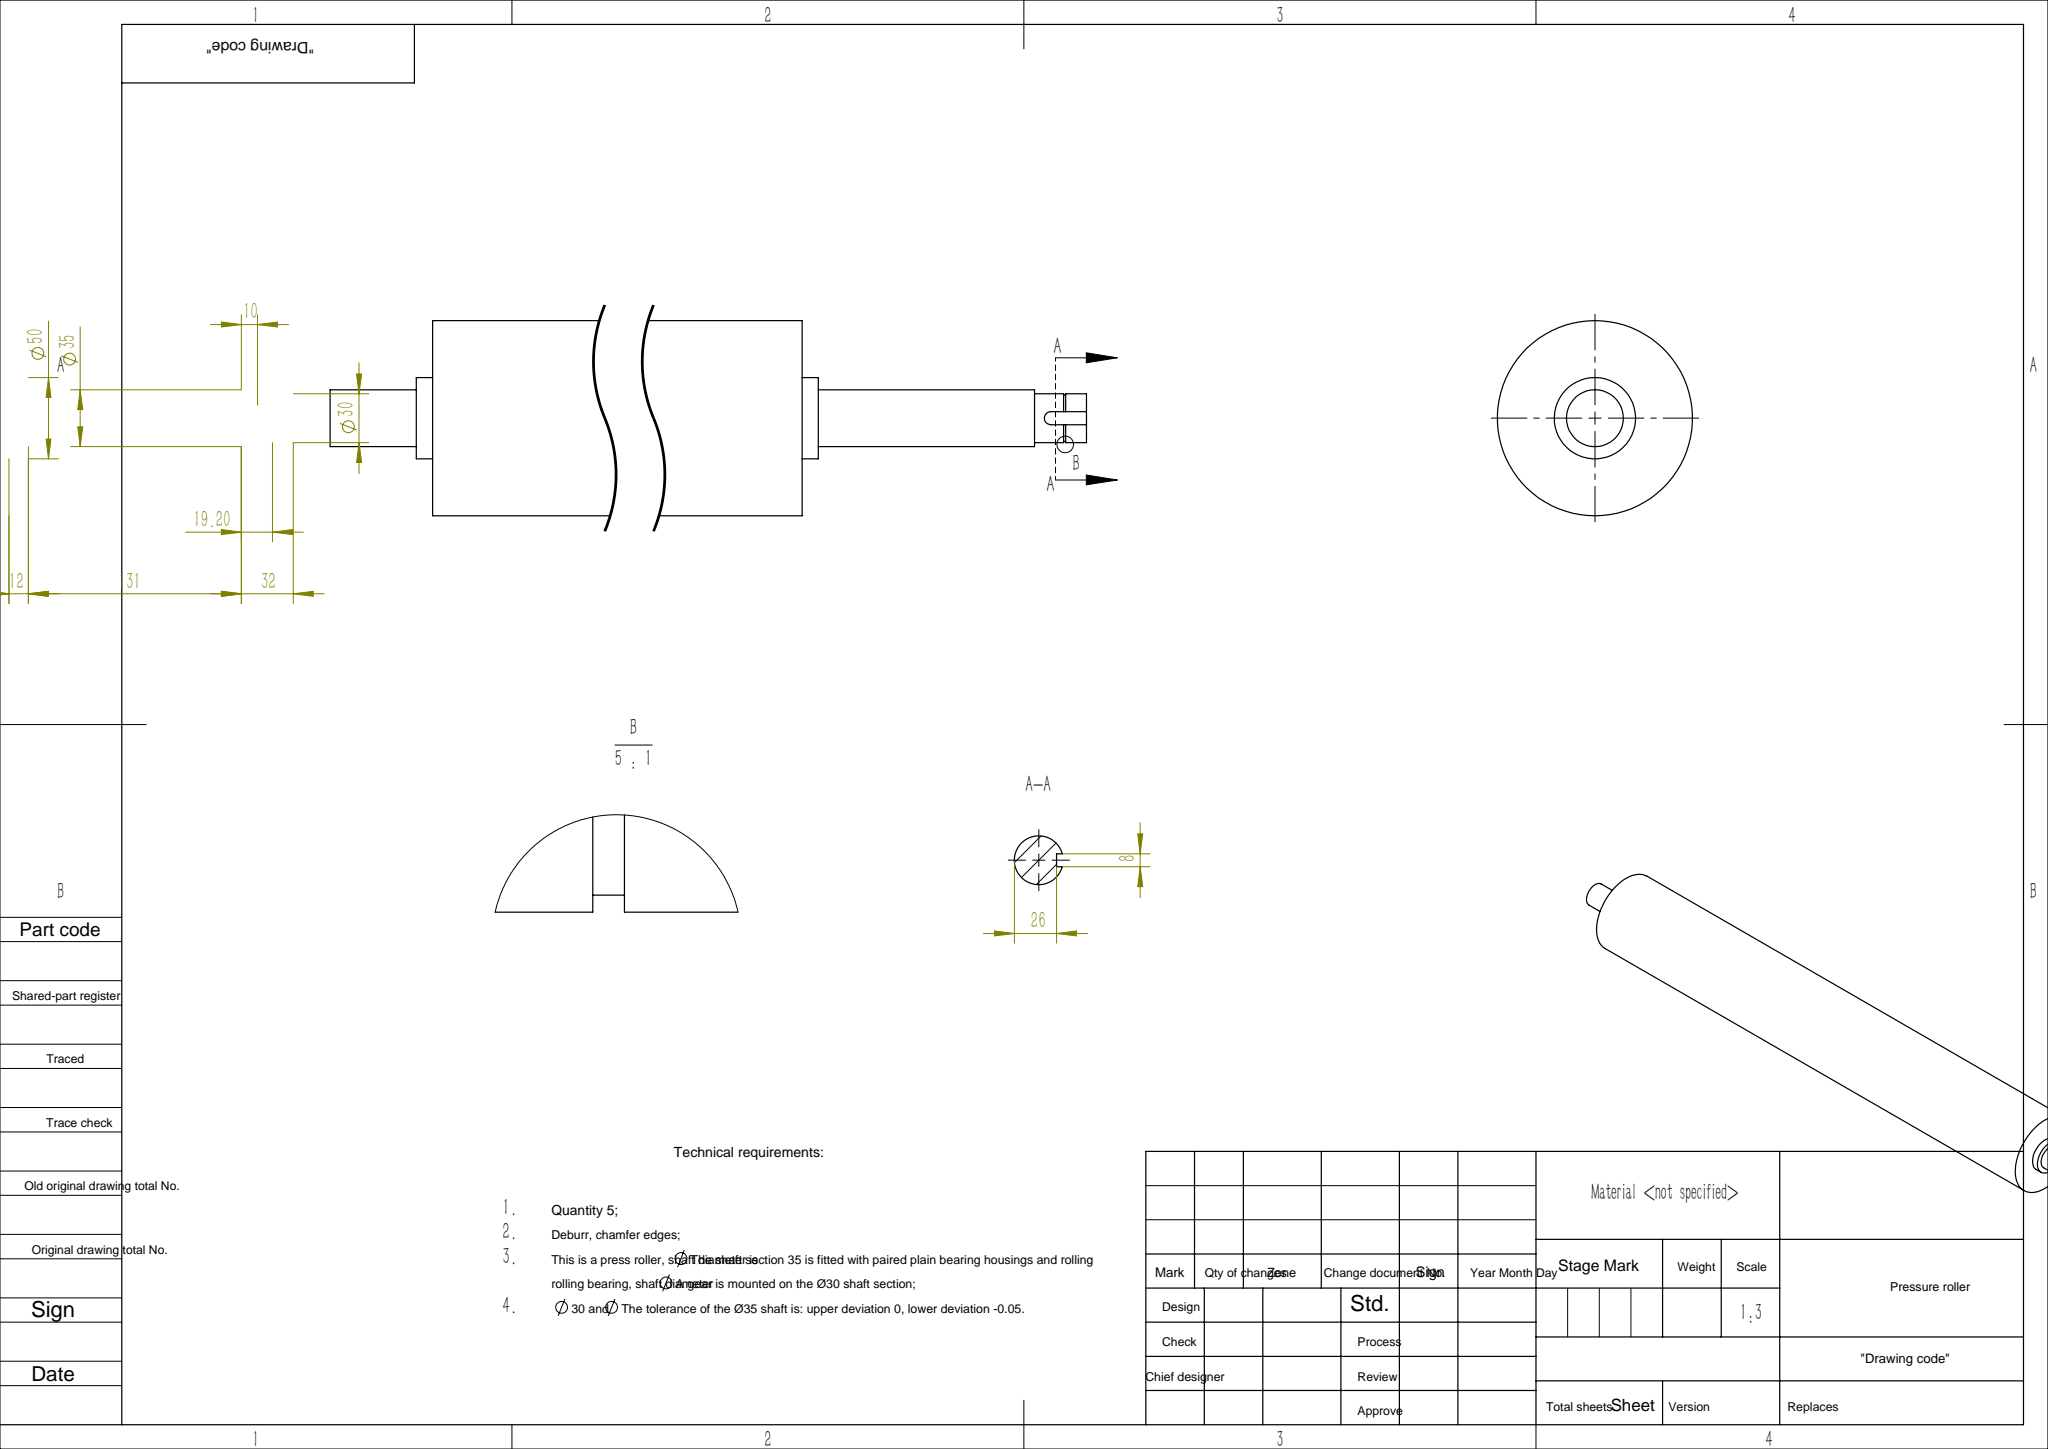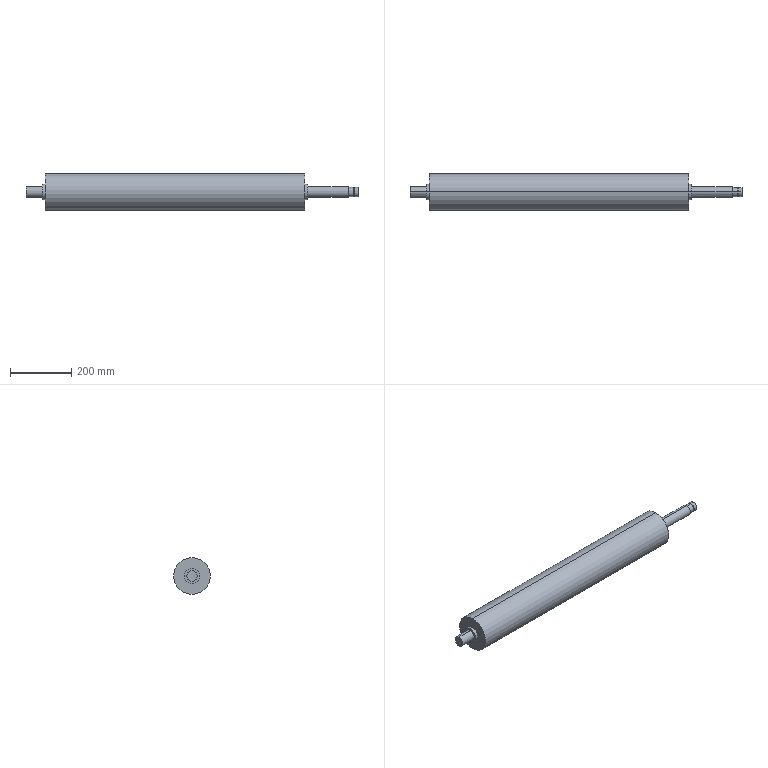Part | SolidWorks | features ICE 2, Revolution 1 | 1 solid | 31 faces | box 1088 x 120 x 120 mm | volume 9853270 mm3 | cylinder 19 | plane 12 | commonest cylinder face diameters 30 x5 35 x4 50 x4 28.6 x3 120 x2 8 x1
STEP:
#1=CARTESIAN_POINT('',(1073.9,13.729,4.));
#2=VERTEX_POINT('',#1);
#3=CARTESIAN_POINT('',(1073.9,0.,14.3));
#4=VERTEX_POINT('',#3);
#5=CARTESIAN_POINT('',(1073.9,0.,0.));
#6=DIRECTION('',(1.,0.,0.));
#7=DIRECTION('',(0.,0.,-1.));
#8=AXIS2_PLACEMENT_3D('',#5,#6,#7);
#9=CIRCLE('',#8,14.3);
#10=EDGE_CURVE('',#2,#4,#9,.T.);
#11=ORIENTED_EDGE('',*,*,#10,.T.);
#12=CARTESIAN_POINT('',(1075.2,0.,14.3));
#13=VERTEX_POINT('',#12);
#14=CARTESIAN_POINT('',(1073.9,0.,14.3));
#15=DIRECTION('',(1.,0.,0.));
#16=VECTOR('',#15,1000.);
#17=LINE('',#14,#16);
#18=EDGE_CURVE('',#4,#13,#17,.T.);
#19=ORIENTED_EDGE('',*,*,#18,.T.);
#20=CARTESIAN_POINT('',(1075.2,13.729,4.));
#21=VERTEX_POINT('',#20);
#22=CARTESIAN_POINT('',(1075.2,0.,0.));
#23=DIRECTION('',(1.,0.,0.));
#24=DIRECTION('',(0.,0.,-1.));
#25=AXIS2_PLACEMENT_3D('',#22,#23,#24);
#26=CIRCLE('',#25,14.3);
#27=EDGE_CURVE('',#21,#13,#26,.T.);
#28=ORIENTED_EDGE('',*,*,#27,.F.);
#29=CARTESIAN_POINT('',(1073.9,13.729,4.));
#30=DIRECTION('',(-1.,0.,0.));
#31=VECTOR('',#30,1000.);
#32=LINE('',#29,#31);
#33=EDGE_CURVE('',#21,#2,#32,.T.);
#34=ORIENTED_EDGE('',*,*,#33,.T.);
#35=EDGE_LOOP('',(#11,#19,#28,#34));
#36=FACE_OUTER_BOUND('',#35,.T.);
#37=CARTESIAN_POINT('',(1073.9,0.,0.));
#38=DIRECTION('',(1.,0.,0.));
#39=DIRECTION('',(0.,0.,-1.));
#40=AXIS2_PLACEMENT_3D('',#37,#38,#39);
#41=CYLINDRICAL_SURFACE('',#40,14.3);
#42=ADVANCED_FACE('',(#36),#41,.T.);
#43=ORIENTED_EDGE('',*,*,#18,.F.);
#44=CARTESIAN_POINT('',(1073.9,0.,-14.3));
#45=VERTEX_POINT('',#44);
#46=CARTESIAN_POINT('',(1073.9,0.,0.));
#47=DIRECTION('',(1.,0.,0.));
#48=DIRECTION('',(0.,0.,-1.));
#49=AXIS2_PLACEMENT_3D('',#46,#47,#48);
#50=CIRCLE('',#49,14.3);
#51=EDGE_CURVE('',#4,#45,#50,.T.);
#52=ORIENTED_EDGE('',*,*,#51,.T.);
#53=CARTESIAN_POINT('',(1075.2,0.,-14.3));
#54=VERTEX_POINT('',#53);
#55=CARTESIAN_POINT('',(1073.9,0.,-14.3));
#56=DIRECTION('',(1.,0.,0.));
#57=VECTOR('',#56,1000.);
#58=LINE('',#55,#57);
#59=EDGE_CURVE('',#45,#54,#58,.T.);
#60=ORIENTED_EDGE('',*,*,#59,.T.);
#61=CARTESIAN_POINT('',(1075.2,0.,0.));
#62=DIRECTION('',(1.,0.,0.));
#63=DIRECTION('',(0.,0.,-1.));
#64=AXIS2_PLACEMENT_3D('',#61,#62,#63);
#65=CIRCLE('',#64,14.3);
#66=EDGE_CURVE('',#13,#54,#65,.T.);
#67=ORIENTED_EDGE('',*,*,#66,.F.);
#68=EDGE_LOOP('',(#43,#52,#60,#67));
#69=FACE_OUTER_BOUND('',#68,.T.);
#70=CARTESIAN_POINT('',(1073.9,0.,0.));
#71=DIRECTION('',(1.,0.,0.));
#72=DIRECTION('',(0.,0.,-1.));
#73=AXIS2_PLACEMENT_3D('',#70,#71,#72);
#74=CYLINDRICAL_SURFACE('',#73,14.3);
#75=ADVANCED_FACE('',(#69),#74,.T.);
#76=CARTESIAN_POINT('',(53.,0.,-25.));
#77=VERTEX_POINT('',#76);
#78=CARTESIAN_POINT('',(53.,0.,25.));
#79=VERTEX_POINT('',#78);
#80=CARTESIAN_POINT('',(53.,0.,0.));
#81=DIRECTION('',(1.,0.,0.));
#82=DIRECTION('',(0.,0.,-1.));
#83=AXIS2_PLACEMENT_3D('',#80,#81,#82);
#84=CIRCLE('',#83,25.);
#85=EDGE_CURVE('',#77,#79,#84,.T.);
#86=ORIENTED_EDGE('',*,*,#85,.T.);
#87=CARTESIAN_POINT('',(63.,0.,25.));
#88=VERTEX_POINT('',#87);
#89=CARTESIAN_POINT('',(1088.,0.,25.));
#90=DIRECTION('',(1.,0.,0.));
#91=VECTOR('',#90,1000.);
#92=LINE('',#89,#91);
#93=EDGE_CURVE('',#79,#88,#92,.T.);
#94=ORIENTED_EDGE('',*,*,#93,.T.);
#95=CARTESIAN_POINT('',(63.,0.,-25.));
#96=VERTEX_POINT('',#95);
#97=CARTESIAN_POINT('',(63.,0.,0.));
#98=DIRECTION('',(1.,0.,0.));
#99=DIRECTION('',(0.,0.,-1.));
#100=AXIS2_PLACEMENT_3D('',#97,#98,#99);
#101=CIRCLE('',#100,25.);
#102=EDGE_CURVE('',#96,#88,#101,.T.);
#103=ORIENTED_EDGE('',*,*,#102,.F.);
#104=CARTESIAN_POINT('',(1088.,0.,-25.));
#105=DIRECTION('',(1.,0.,0.));
#106=VECTOR('',#105,1000.);
#107=LINE('',#104,#106);
#108=EDGE_CURVE('',#77,#96,#107,.T.);
#109=ORIENTED_EDGE('',*,*,#108,.F.);
#110=EDGE_LOOP('',(#86,#94,#103,#109));
#111=FACE_OUTER_BOUND('',#110,.T.);
#112=CARTESIAN_POINT('',(1088.,0.,0.));
#113=DIRECTION('',(1.,0.,0.));
#114=DIRECTION('',(0.,0.,-1.));
#115=AXIS2_PLACEMENT_3D('',#112,#113,#114);
#116=CYLINDRICAL_SURFACE('',#115,25.);
#117=ADVANCED_FACE('',(#111),#116,.T.);
#118=CARTESIAN_POINT('',(63.,0.,-60.));
#119=VERTEX_POINT('',#118);
#120=CARTESIAN_POINT('',(63.,0.,60.));
#121=VERTEX_POINT('',#120);
#122=CARTESIAN_POINT('',(63.,0.,0.));
#123=DIRECTION('',(1.,0.,0.));
#124=DIRECTION('',(0.,0.,-1.));
#125=AXIS2_PLACEMENT_3D('',#122,#123,#124);
#126=CIRCLE('',#125,60.);
#127=EDGE_CURVE('',#119,#121,#126,.T.);
#128=ORIENTED_EDGE('',*,*,#127,.T.);
#129=CARTESIAN_POINT('',(913.,0.,60.));
#130=VERTEX_POINT('',#129);
#131=CARTESIAN_POINT('',(1088.,0.,60.));
#132=DIRECTION('',(1.,0.,0.));
#133=VECTOR('',#132,1000.);
#134=LINE('',#131,#133);
#135=EDGE_CURVE('',#121,#130,#134,.T.);
#136=ORIENTED_EDGE('',*,*,#135,.T.);
#137=CARTESIAN_POINT('',(913.,0.,-60.));
#138=VERTEX_POINT('',#137);
#139=CARTESIAN_POINT('',(913.,0.,0.));
#140=DIRECTION('',(1.,0.,0.));
#141=DIRECTION('',(0.,0.,-1.));
#142=AXIS2_PLACEMENT_3D('',#139,#140,#141);
#143=CIRCLE('',#142,60.);
#144=EDGE_CURVE('',#138,#130,#143,.T.);
#145=ORIENTED_EDGE('',*,*,#144,.F.);
#146=CARTESIAN_POINT('',(1088.,0.,-60.));
#147=DIRECTION('',(1.,0.,0.));
#148=VECTOR('',#147,1000.);
#149=LINE('',#146,#148);
#150=EDGE_CURVE('',#119,#138,#149,.T.);
#151=ORIENTED_EDGE('',*,*,#150,.F.);
#152=EDGE_LOOP('',(#128,#136,#145,#151));
#153=FACE_OUTER_BOUND('',#152,.T.);
#154=CARTESIAN_POINT('',(1088.,0.,0.));
#155=DIRECTION('',(1.,0.,0.));
#156=DIRECTION('',(0.,0.,-1.));
#157=AXIS2_PLACEMENT_3D('',#154,#155,#156);
#158=CYLINDRICAL_SURFACE('',#157,60.);
#159=ADVANCED_FACE('',(#153),#158,.T.);
#160=CARTESIAN_POINT('',(913.,0.,-25.));
#161=VERTEX_POINT('',#160);
#162=CARTESIAN_POINT('',(913.,0.,25.));
#163=VERTEX_POINT('',#162);
#164=CARTESIAN_POINT('',(913.,0.,0.));
#165=DIRECTION('',(1.,0.,0.));
#166=DIRECTION('',(0.,0.,-1.));
#167=AXIS2_PLACEMENT_3D('',#164,#165,#166);
#168=CIRCLE('',#167,25.);
#169=EDGE_CURVE('',#161,#163,#168,.T.);
#170=ORIENTED_EDGE('',*,*,#169,.T.);
#171=CARTESIAN_POINT('',(923.,0.,25.));
#172=VERTEX_POINT('',#171);
#173=CARTESIAN_POINT('',(1088.,0.,25.));
#174=DIRECTION('',(1.,0.,0.));
#175=VECTOR('',#174,1000.);
#176=LINE('',#173,#175);
#177=EDGE_CURVE('',#163,#172,#176,.T.);
#178=ORIENTED_EDGE('',*,*,#177,.T.);
#179=CARTESIAN_POINT('',(923.,0.,-25.));
#180=VERTEX_POINT('',#179);
#181=CARTESIAN_POINT('',(923.,0.,0.));
#182=DIRECTION('',(1.,0.,0.));
#183=DIRECTION('',(0.,0.,-1.));
#184=AXIS2_PLACEMENT_3D('',#181,#182,#183);
#185=CIRCLE('',#184,25.);
#186=EDGE_CURVE('',#180,#172,#185,.T.);
#187=ORIENTED_EDGE('',*,*,#186,.F.);
#188=CARTESIAN_POINT('',(1088.,0.,-25.));
#189=DIRECTION('',(1.,0.,0.));
#190=VECTOR('',#189,1000.);
#191=LINE('',#188,#190);
#192=EDGE_CURVE('',#161,#180,#191,.T.);
#193=ORIENTED_EDGE('',*,*,#192,.F.);
#194=EDGE_LOOP('',(#170,#178,#187,#193));
#195=FACE_OUTER_BOUND('',#194,.T.);
#196=CARTESIAN_POINT('',(1088.,0.,0.));
#197=DIRECTION('',(1.,0.,0.));
#198=DIRECTION('',(0.,0.,-1.));
#199=AXIS2_PLACEMENT_3D('',#196,#197,#198);
#200=CYLINDRICAL_SURFACE('',#199,25.);
#201=ADVANCED_FACE('',(#195),#200,.T.);
#202=CARTESIAN_POINT('',(923.,0.,-17.5));
#203=VERTEX_POINT('',#202);
#204=CARTESIAN_POINT('',(923.,0.,17.5));
#205=VERTEX_POINT('',#204);
#206=CARTESIAN_POINT('',(923.,0.,0.));
#207=DIRECTION('',(1.,0.,0.));
#208=DIRECTION('',(0.,0.,-1.));
#209=AXIS2_PLACEMENT_3D('',#206,#207,#208);
#210=CIRCLE('',#209,17.5);
#211=EDGE_CURVE('',#203,#205,#210,.T.);
#212=ORIENTED_EDGE('',*,*,#211,.T.);
#213=CARTESIAN_POINT('',(1056.,0.,17.5));
#214=VERTEX_POINT('',#213);
#215=CARTESIAN_POINT('',(1088.,0.,17.5));
#216=DIRECTION('',(1.,0.,0.));
#217=VECTOR('',#216,1000.);
#218=LINE('',#215,#217);
#219=EDGE_CURVE('',#205,#214,#218,.T.);
#220=ORIENTED_EDGE('',*,*,#219,.T.);
#221=CARTESIAN_POINT('',(1056.,0.,-17.5));
#222=VERTEX_POINT('',#221);
#223=CARTESIAN_POINT('',(1056.,0.,0.));
#224=DIRECTION('',(1.,0.,0.));
#225=DIRECTION('',(0.,0.,-1.));
#226=AXIS2_PLACEMENT_3D('',#223,#224,#225);
#227=CIRCLE('',#226,17.5);
#228=EDGE_CURVE('',#222,#214,#227,.T.);
#229=ORIENTED_EDGE('',*,*,#228,.F.);
#230=CARTESIAN_POINT('',(1088.,0.,-17.5));
#231=DIRECTION('',(1.,0.,0.));
#232=VECTOR('',#231,1000.);
#233=LINE('',#230,#232);
#234=EDGE_CURVE('',#203,#222,#233,.T.);
#235=ORIENTED_EDGE('',*,*,#234,.F.);
#236=EDGE_LOOP('',(#212,#220,#229,#235));
#237=FACE_OUTER_BOUND('',#236,.T.);
#238=CARTESIAN_POINT('',(1088.,0.,0.));
#239=DIRECTION('',(1.,0.,0.));
#240=DIRECTION('',(0.,0.,-1.));
#241=AXIS2_PLACEMENT_3D('',#238,#239,#240);
#242=CYLINDRICAL_SURFACE('',#241,17.5);
#243=ADVANCED_FACE('',(#237),#242,.T.);
#244=CARTESIAN_POINT('',(1075.2,14.457,4.));
#245=VERTEX_POINT('',#244);
#246=CARTESIAN_POINT('',(1075.2,0.,15.));
#247=VERTEX_POINT('',#246);
#248=CARTESIAN_POINT('',(1075.2,0.,0.));
#249=DIRECTION('',(1.,0.,0.));
#250=DIRECTION('',(0.,0.,-1.));
#251=AXIS2_PLACEMENT_3D('',#248,#249,#250);
#252=CIRCLE('',#251,15.);
#253=EDGE_CURVE('',#245,#247,#252,.T.);
#254=ORIENTED_EDGE('',*,*,#253,.T.);
#255=CARTESIAN_POINT('',(1088.,0.,15.));
#256=VERTEX_POINT('',#255);
#257=CARTESIAN_POINT('',(1088.,0.,15.));
#258=DIRECTION('',(1.,0.,0.));
#259=VECTOR('',#258,1000.);
#260=LINE('',#257,#259);
#261=EDGE_CURVE('',#247,#256,#260,.T.);
#262=ORIENTED_EDGE('',*,*,#261,.T.);
#263=CARTESIAN_POINT('',(1088.,14.457,4.));
#264=VERTEX_POINT('',#263);
#265=CARTESIAN_POINT('',(1088.,0.,0.));
#266=DIRECTION('',(1.,0.,0.));
#267=DIRECTION('',(0.,0.,-1.));
#268=AXIS2_PLACEMENT_3D('',#265,#266,#267);
#269=CIRCLE('',#268,15.);
#270=EDGE_CURVE('',#264,#256,#269,.T.);
#271=ORIENTED_EDGE('',*,*,#270,.F.);
#272=CARTESIAN_POINT('',(1088.,14.457,4.));
#273=DIRECTION('',(1.,0.,0.));
#274=VECTOR('',#273,1000.);
#275=LINE('',#272,#274);
#276=EDGE_CURVE('',#245,#264,#275,.T.);
#277=ORIENTED_EDGE('',*,*,#276,.F.);
#278=EDGE_LOOP('',(#254,#262,#271,#277));
#279=FACE_OUTER_BOUND('',#278,.T.);
#280=CARTESIAN_POINT('',(1088.,0.,0.));
#281=DIRECTION('',(1.,0.,0.));
#282=DIRECTION('',(0.,0.,-1.));
#283=AXIS2_PLACEMENT_3D('',#280,#281,#282);
#284=CYLINDRICAL_SURFACE('',#283,15.);
#285=ADVANCED_FACE('',(#279),#284,.T.);
#286=ORIENTED_EDGE('',*,*,#261,.F.);
#287=CARTESIAN_POINT('',(1075.2,0.,-15.));
#288=VERTEX_POINT('',#287);
#289=CARTESIAN_POINT('',(1075.2,0.,0.));
#290=DIRECTION('',(1.,0.,0.));
#291=DIRECTION('',(0.,0.,-1.));
#292=AXIS2_PLACEMENT_3D('',#289,#290,#291);
#293=CIRCLE('',#292,15.);
#294=EDGE_CURVE('',#247,#288,#293,.T.);
#295=ORIENTED_EDGE('',*,*,#294,.T.);
#296=CARTESIAN_POINT('',(1088.,0.,-15.));
#297=VERTEX_POINT('',#296);
#298=CARTESIAN_POINT('',(1088.,0.,-15.));
#299=DIRECTION('',(1.,0.,0.));
#300=VECTOR('',#299,1000.);
#301=LINE('',#298,#300);
#302=EDGE_CURVE('',#288,#297,#301,.T.);
#303=ORIENTED_EDGE('',*,*,#302,.T.);
#304=CARTESIAN_POINT('',(1088.,0.,0.));
#305=DIRECTION('',(1.,0.,0.));
#306=DIRECTION('',(0.,0.,-1.));
#307=AXIS2_PLACEMENT_3D('',#304,#305,#306);
#308=CIRCLE('',#307,15.);
#309=EDGE_CURVE('',#256,#297,#308,.T.);
#310=ORIENTED_EDGE('',*,*,#309,.F.);
#311=EDGE_LOOP('',(#286,#295,#303,#310));
#312=FACE_OUTER_BOUND('',#311,.T.);
#313=CARTESIAN_POINT('',(1088.,0.,0.));
#314=DIRECTION('',(1.,0.,0.));
#315=DIRECTION('',(0.,0.,-1.));
#316=AXIS2_PLACEMENT_3D('',#313,#314,#315);
#317=CYLINDRICAL_SURFACE('',#316,15.);
#318=ADVANCED_FACE('',(#312),#317,.T.);
#319=CARTESIAN_POINT('',(0.,0.,-17.5));
#320=VERTEX_POINT('',#319);
#321=CARTESIAN_POINT('',(0.,0.,17.5));
#322=VERTEX_POINT('',#321);
#323=CARTESIAN_POINT('',(0.,0.,0.));
#324=DIRECTION('',(1.,0.,0.));
#325=DIRECTION('',(0.,0.,-1.));
#326=AXIS2_PLACEMENT_3D('',#323,#324,#325);
#327=CIRCLE('',#326,17.5);
#328=EDGE_CURVE('',#320,#322,#327,.T.);
#329=ORIENTED_EDGE('',*,*,#328,.T.);
#330=CARTESIAN_POINT('',(53.,0.,17.5));
#331=VERTEX_POINT('',#330);
#332=CARTESIAN_POINT('',(1088.,0.,17.5));
#333=DIRECTION('',(1.,0.,0.));
#334=VECTOR('',#333,1000.);
#335=LINE('',#332,#334);
#336=EDGE_CURVE('',#322,#331,#335,.T.);
#337=ORIENTED_EDGE('',*,*,#336,.T.);
#338=CARTESIAN_POINT('',(53.,0.,-17.5));
#339=VERTEX_POINT('',#338);
#340=CARTESIAN_POINT('',(53.,0.,0.));
#341=DIRECTION('',(1.,0.,0.));
#342=DIRECTION('',(0.,0.,-1.));
#343=AXIS2_PLACEMENT_3D('',#340,#341,#342);
#344=CIRCLE('',#343,17.5);
#345=EDGE_CURVE('',#339,#331,#344,.T.);
#346=ORIENTED_EDGE('',*,*,#345,.F.);
#347=CARTESIAN_POINT('',(1088.,0.,-17.5));
#348=DIRECTION('',(1.,0.,0.));
#349=VECTOR('',#348,1000.);
#350=LINE('',#347,#349);
#351=EDGE_CURVE('',#320,#339,#350,.T.);
#352=ORIENTED_EDGE('',*,*,#351,.F.);
#353=EDGE_LOOP('',(#329,#337,#346,#352));
#354=FACE_OUTER_BOUND('',#353,.T.);
#355=CARTESIAN_POINT('',(1088.,0.,0.));
#356=DIRECTION('',(1.,0.,0.));
#357=DIRECTION('',(0.,0.,-1.));
#358=AXIS2_PLACEMENT_3D('',#355,#356,#357);
#359=CYLINDRICAL_SURFACE('',#358,17.5);
#360=ADVANCED_FACE('',(#354),#359,.T.);
#361=CARTESIAN_POINT('',(1056.,0.,-15.));
#362=VERTEX_POINT('',#361);
#363=CARTESIAN_POINT('',(1056.,0.,15.));
#364=VERTEX_POINT('',#363);
#365=CARTESIAN_POINT('',(1056.,0.,0.));
#366=DIRECTION('',(1.,0.,0.));
#367=DIRECTION('',(0.,0.,-1.));
#368=AXIS2_PLACEMENT_3D('',#365,#366,#367);
#369=CIRCLE('',#368,15.);
#370=EDGE_CURVE('',#362,#364,#369,.T.);
#371=ORIENTED_EDGE('',*,*,#370,.T.);
#372=CARTESIAN_POINT('',(1073.9,0.,15.));
#373=VERTEX_POINT('',#372);
#374=CARTESIAN_POINT('',(1088.,0.,15.));
#375=DIRECTION('',(1.,0.,0.));
#376=VECTOR('',#375,1000.);
#377=LINE('',#374,#376);
#378=EDGE_CURVE('',#364,#373,#377,.T.);
#379=ORIENTED_EDGE('',*,*,#378,.T.);
#380=CARTESIAN_POINT('',(1073.9,14.457,4.));
#381=VERTEX_POINT('',#380);
#382=CARTESIAN_POINT('',(1073.9,0.,0.));
#383=DIRECTION('',(1.,0.,0.));
#384=DIRECTION('',(0.,0.,-1.));
#385=AXIS2_PLACEMENT_3D('',#382,#383,#384);
#386=CIRCLE('',#385,15.);
#387=EDGE_CURVE('',#381,#373,#386,.T.);
#388=ORIENTED_EDGE('',*,*,#387,.F.);
#389=CARTESIAN_POINT('',(1066.,14.457,4.));
#390=VERTEX_POINT('',#389);
#391=CARTESIAN_POINT('',(1088.,14.457,4.));
#392=DIRECTION('',(1.,0.,0.));
#393=VECTOR('',#392,1000.);
#394=LINE('',#391,#393);
#395=EDGE_CURVE('',#390,#381,#394,.T.);
#396=ORIENTED_EDGE('',*,*,#395,.F.);
#397=CARTESIAN_POINT('',(1066.,14.457,-4.));
#398=VERTEX_POINT('',#397);
#399=CARTESIAN_POINT('',(1066.,14.457,-4.));
#400=CARTESIAN_POINT('',(1065.734,14.457,-4.));
#401=CARTESIAN_POINT('',(1065.474,14.464,-3.974));
#402=CARTESIAN_POINT('',(1064.961,14.492,-3.872));
#403=CARTESIAN_POINT('',(1064.706,14.513,-3.794));
#404=CARTESIAN_POINT('',(1064.223,14.564,-3.593));
#405=CARTESIAN_POINT('',(1063.993,14.594,-3.47));
#406=CARTESIAN_POINT('',(1063.56,14.66,-3.18));
#407=CARTESIAN_POINT('',(1063.355,14.696,-3.012));
#408=CARTESIAN_POINT('',(1062.988,14.766,-2.645));
#409=CARTESIAN_POINT('',(1062.823,14.801,-2.444));
#410=CARTESIAN_POINT('',(1062.53,14.867,-2.008));
#411=CARTESIAN_POINT('',(1062.407,14.896,-1.777));
#412=CARTESIAN_POINT('',(1062.207,14.946,-1.296));
#413=CARTESIAN_POINT('',(1062.129,14.966,-1.043));
#414=CARTESIAN_POINT('',(1062.026,14.993,-0.5261));
#415=CARTESIAN_POINT('',(1062.,15.,-0.2658));
#416=CARTESIAN_POINT('',(1062.,15.,0.2585));
#417=CARTESIAN_POINT('',(1062.026,14.993,0.5249));
#418=CARTESIAN_POINT('',(1062.128,14.966,1.039));
#419=CARTESIAN_POINT('',(1062.204,14.947,1.289));
#420=CARTESIAN_POINT('',(1062.506,14.872,2.017));
#421=CARTESIAN_POINT('',(1062.801,14.802,2.457));
#422=CARTESIAN_POINT('',(1063.355,14.696,3.012));
#423=CARTESIAN_POINT('',(1063.556,14.66,3.177));
#424=CARTESIAN_POINT('',(1063.988,14.595,3.467));
#425=CARTESIAN_POINT('',(1064.222,14.564,3.593));
#426=CARTESIAN_POINT('',(1064.704,14.513,3.793));
#427=CARTESIAN_POINT('',(1064.954,14.492,3.87));
#428=CARTESIAN_POINT('',(1065.469,14.464,3.973));
#429=CARTESIAN_POINT('',(1065.734,14.457,4.));
#430=CARTESIAN_POINT('',(1066.,14.457,4.));
#431=B_SPLINE_CURVE_WITH_KNOTS('',3,(#399,#400,#401,#402,#403,#404,#405,#406,#407,#408,#409,#410,#411,#412,#413,#414,#415,#416,#417,#418,#419,#420,#421,#422,#423,#424,#425,#426,#427,#428,#429,#430),.UNSPECIFIED.,.F.,.F.,(4,2,2,2,2,2,2,2,2,2,2,2,2,2,2,4),(0.,0.0007849,0.00157,0.002355,0.00314,0.003925,0.00471,0.005494,0.006279,0.007064,0.007849,0.009419,0.0102,0.01099,0.01177,0.01256),.UNSPECIFIED.);
#432=EDGE_CURVE('',#398,#390,#431,.T.);
#433=ORIENTED_EDGE('',*,*,#432,.F.);
#434=CARTESIAN_POINT('',(1073.9,14.457,-4.));
#435=VERTEX_POINT('',#434);
#436=CARTESIAN_POINT('',(1088.,14.457,-4.));
#437=DIRECTION('',(-1.,0.,0.));
#438=VECTOR('',#437,1000.);
#439=LINE('',#436,#438);
#440=EDGE_CURVE('',#435,#398,#439,.T.);
#441=ORIENTED_EDGE('',*,*,#440,.F.);
#442=CARTESIAN_POINT('',(1073.9,0.,-15.));
#443=VERTEX_POINT('',#442);
#444=CARTESIAN_POINT('',(1073.9,0.,0.));
#445=DIRECTION('',(1.,0.,0.));
#446=DIRECTION('',(0.,0.,-1.));
#447=AXIS2_PLACEMENT_3D('',#444,#445,#446);
#448=CIRCLE('',#447,15.);
#449=EDGE_CURVE('',#443,#435,#448,.T.);
#450=ORIENTED_EDGE('',*,*,#449,.F.);
#451=CARTESIAN_POINT('',(1088.,0.,-15.));
#452=DIRECTION('',(1.,0.,0.));
#453=VECTOR('',#452,1000.);
#454=LINE('',#451,#453);
#455=EDGE_CURVE('',#362,#443,#454,.T.);
#456=ORIENTED_EDGE('',*,*,#455,.F.);
#457=EDGE_LOOP('',(#371,#379,#388,#396,#433,#441,#450,#456));
#458=FACE_OUTER_BOUND('',#457,.T.);
#459=CARTESIAN_POINT('',(1088.,0.,0.));
#460=DIRECTION('',(1.,0.,0.));
#461=DIRECTION('',(0.,0.,-1.));
#462=AXIS2_PLACEMENT_3D('',#459,#460,#461);
#463=CYLINDRICAL_SURFACE('',#462,15.);
#464=ADVANCED_FACE('',(#458),#463,.T.);
#465=ORIENTED_EDGE('',*,*,#378,.F.);
#466=CARTESIAN_POINT('',(1056.,0.,0.));
#467=DIRECTION('',(1.,0.,0.));
#468=DIRECTION('',(0.,0.,-1.));
#469=AXIS2_PLACEMENT_3D('',#466,#467,#468);
#470=CIRCLE('',#469,15.);
#471=EDGE_CURVE('',#364,#362,#470,.T.);
#472=ORIENTED_EDGE('',*,*,#471,.T.);
#473=ORIENTED_EDGE('',*,*,#455,.T.);
#474=CARTESIAN_POINT('',(1073.9,0.,0.));
#475=DIRECTION('',(1.,0.,0.));
#476=DIRECTION('',(0.,0.,-1.));
#477=AXIS2_PLACEMENT_3D('',#474,#475,#476);
#478=CIRCLE('',#477,15.);
#479=EDGE_CURVE('',#373,#443,#478,.T.);
#480=ORIENTED_EDGE('',*,*,#479,.F.);
#481=EDGE_LOOP('',(#465,#472,#473,#480));
#482=FACE_OUTER_BOUND('',#481,.T.);
#483=CARTESIAN_POINT('',(1088.,0.,0.));
#484=DIRECTION('',(1.,0.,0.));
#485=DIRECTION('',(0.,0.,-1.));
#486=AXIS2_PLACEMENT_3D('',#483,#484,#485);
#487=CYLINDRICAL_SURFACE('',#486,15.);
#488=ADVANCED_FACE('',(#482),#487,.T.);
#489=CARTESIAN_POINT('',(1073.9,13.729,-4.));
#490=VERTEX_POINT('',#489);
#491=CARTESIAN_POINT('',(1073.9,11.,-4.));
#492=DIRECTION('',(0.,-1.,0.));
#493=VECTOR('',#492,1000.);
#494=LINE('',#491,#493);
#495=EDGE_CURVE('',#435,#490,#494,.T.);
#496=ORIENTED_EDGE('',*,*,#495,.F.);
#497=ORIENTED_EDGE('',*,*,#440,.T.);
#498=CARTESIAN_POINT('',(1066.,11.,-4.));
#499=VERTEX_POINT('',#498);
#500=CARTESIAN_POINT('',(1066.,11.,-4.));
#501=DIRECTION('',(0.,1.,0.));
#502=VECTOR('',#501,1000.);
#503=LINE('',#500,#502);
#504=EDGE_CURVE('',#499,#398,#503,.T.);
#505=ORIENTED_EDGE('',*,*,#504,.F.);
#506=CARTESIAN_POINT('',(1088.,11.,-4.));
#507=VERTEX_POINT('',#506);
#508=CARTESIAN_POINT('',(1066.,11.,-4.));
#509=DIRECTION('',(-1.,0.,0.));
#510=VECTOR('',#509,1000.);
#511=LINE('',#508,#510);
#512=EDGE_CURVE('',#507,#499,#511,.T.);
#513=ORIENTED_EDGE('',*,*,#512,.F.);
#514=CARTESIAN_POINT('',(1088.,14.457,-4.));
#515=VERTEX_POINT('',#514);
#516=CARTESIAN_POINT('',(1088.,15.,-4.));
#517=DIRECTION('',(0.,1.,0.));
#518=VECTOR('',#517,1000.);
#519=LINE('',#516,#518);
#520=EDGE_CURVE('',#507,#515,#519,.T.);
#521=ORIENTED_EDGE('',*,*,#520,.T.);
#522=CARTESIAN_POINT('',(1075.2,14.457,-4.));
#523=VERTEX_POINT('',#522);
#524=CARTESIAN_POINT('',(1088.,14.457,-4.));
#525=DIRECTION('',(-1.,0.,0.));
#526=VECTOR('',#525,1000.);
#527=LINE('',#524,#526);
#528=EDGE_CURVE('',#515,#523,#527,.T.);
#529=ORIENTED_EDGE('',*,*,#528,.T.);
#530=CARTESIAN_POINT('',(1075.2,13.729,-4.));
#531=VERTEX_POINT('',#530);
#532=CARTESIAN_POINT('',(1075.2,11.,-4.));
#533=DIRECTION('',(0.,-1.,0.));
#534=VECTOR('',#533,1000.);
#535=LINE('',#532,#534);
#536=EDGE_CURVE('',#523,#531,#535,.T.);
#537=ORIENTED_EDGE('',*,*,#536,.T.);
#538=CARTESIAN_POINT('',(1073.9,13.729,-4.));
#539=DIRECTION('',(1.,0.,0.));
#540=VECTOR('',#539,1000.);
#541=LINE('',#538,#540);
#542=EDGE_CURVE('',#490,#531,#541,.T.);
#543=ORIENTED_EDGE('',*,*,#542,.F.);
#544=EDGE_LOOP('',(#496,#497,#505,#513,#521,#529,#537,#543));
#545=FACE_OUTER_BOUND('',#544,.T.);
#546=CARTESIAN_POINT('',(1066.,11.,-4.));
#547=DIRECTION('',(0.,0.,-1.));
#548=DIRECTION('',(-1.,0.,0.));
#549=AXIS2_PLACEMENT_3D('',#546,#547,#548);
#550=PLANE('',#549);
#551=ADVANCED_FACE('',(#545),#550,.F.);
#552=CARTESIAN_POINT('',(1073.9,11.,4.));
#553=DIRECTION('',(0.,1.,0.));
#554=VECTOR('',#553,1000.);
#555=LINE('',#552,#554);
#556=EDGE_CURVE('',#2,#381,#555,.T.);
#557=ORIENTED_EDGE('',*,*,#556,.F.);
#558=ORIENTED_EDGE('',*,*,#33,.F.);
#559=CARTESIAN_POINT('',(1075.2,11.,4.));
#560=DIRECTION('',(0.,1.,0.));
#561=VECTOR('',#560,1000.);
#562=LINE('',#559,#561);
#563=EDGE_CURVE('',#21,#245,#562,.T.);
#564=ORIENTED_EDGE('',*,*,#563,.T.);
#565=ORIENTED_EDGE('',*,*,#276,.T.);
#566=CARTESIAN_POINT('',(1088.,11.,4.));
#567=VERTEX_POINT('',#566);
#568=CARTESIAN_POINT('',(1088.,15.,4.));
#569=DIRECTION('',(0.,-1.,0.));
#570=VECTOR('',#569,1000.);
#571=LINE('',#568,#570);
#572=EDGE_CURVE('',#264,#567,#571,.T.);
#573=ORIENTED_EDGE('',*,*,#572,.T.);
#574=CARTESIAN_POINT('',(1066.,11.,4.));
#575=VERTEX_POINT('',#574);
#576=CARTESIAN_POINT('',(1098.,11.,4.));
#577=DIRECTION('',(1.,0.,0.));
#578=VECTOR('',#577,1000.);
#579=LINE('',#576,#578);
#580=EDGE_CURVE('',#575,#567,#579,.T.);
#581=ORIENTED_EDGE('',*,*,#580,.F.);
#582=CARTESIAN_POINT('',(1066.,11.,4.));
#583=DIRECTION('',(0.,1.,0.));
#584=VECTOR('',#583,1000.);
#585=LINE('',#582,#584);
#586=EDGE_CURVE('',#575,#390,#585,.T.);
#587=ORIENTED_EDGE('',*,*,#586,.T.);
#588=ORIENTED_EDGE('',*,*,#395,.T.);
#589=EDGE_LOOP('',(#557,#558,#564,#565,#573,#581,#587,#588));
#590=FACE_OUTER_BOUND('',#589,.T.);
#591=CARTESIAN_POINT('',(1098.,11.,4.));
#592=DIRECTION('',(0.,0.,1.));
#593=DIRECTION('',(1.,0.,0.));
#594=AXIS2_PLACEMENT_3D('',#591,#592,#593);
#595=PLANE('',#594);
#596=ADVANCED_FACE('',(#590),#595,.F.);
#597=ORIENTED_EDGE('',*,*,#336,.F.);
#598=CARTESIAN_POINT('',(0.,0.,0.));
#599=DIRECTION('',(1.,0.,0.));
#600=DIRECTION('',(0.,0.,-1.));
#601=AXIS2_PLACEMENT_3D('',#598,#599,#600);
#602=CIRCLE('',#601,17.5);
#603=EDGE_CURVE('',#322,#320,#602,.T.);
#604=ORIENTED_EDGE('',*,*,#603,.T.);
#605=ORIENTED_EDGE('',*,*,#351,.T.);
#606=CARTESIAN_POINT('',(53.,0.,0.));
#607=DIRECTION('',(1.,0.,0.));
#608=DIRECTION('',(0.,0.,-1.));
#609=AXIS2_PLACEMENT_3D('',#606,#607,#608);
#610=CIRCLE('',#609,17.5);
#611=EDGE_CURVE('',#331,#339,#610,.T.);
#612=ORIENTED_EDGE('',*,*,#611,.F.);
#613=EDGE_LOOP('',(#597,#604,#605,#612));
#614=FACE_OUTER_BOUND('',#613,.T.);
#615=CARTESIAN_POINT('',(1088.,0.,0.));
#616=DIRECTION('',(1.,0.,0.));
#617=DIRECTION('',(0.,0.,-1.));
#618=AXIS2_PLACEMENT_3D('',#615,#616,#617);
#619=CYLINDRICAL_SURFACE('',#618,17.5);
#620=ADVANCED_FACE('',(#614),#619,.T.);
#621=ORIENTED_EDGE('',*,*,#328,.F.);
#622=ORIENTED_EDGE('',*,*,#603,.F.);
#623=EDGE_LOOP('',(#621,#622));
#624=FACE_OUTER_BOUND('',#623,.T.);
#625=CARTESIAN_POINT('',(0.,0.,0.));
#626=DIRECTION('',(-1.,0.,0.));
#627=DIRECTION('',(0.,0.,1.));
#628=AXIS2_PLACEMENT_3D('',#625,#626,#627);
#629=PLANE('',#628);
#630=ADVANCED_FACE('',(#624),#629,.T.);
#631=ORIENTED_EDGE('',*,*,#520,.F.);
#632=CARTESIAN_POINT('',(1088.,11.,0.));
#633=DIRECTION('',(0.,0.,1.));
#634=VECTOR('',#633,1000.);
#635=LINE('',#632,#634);
#636=EDGE_CURVE('',#507,#567,#635,.T.);
#637=ORIENTED_EDGE('',*,*,#636,.T.);
#638=ORIENTED_EDGE('',*,*,#572,.F.);
#639=ORIENTED_EDGE('',*,*,#270,.T.);
#640=ORIENTED_EDGE('',*,*,#309,.T.);
#641=CARTESIAN_POINT('',(1088.,0.,0.));
#642=DIRECTION('',(1.,0.,0.));
#643=DIRECTION('',(0.,0.,-1.));
#644=AXIS2_PLACEMENT_3D('',#641,#642,#643);
#645=CIRCLE('',#644,15.);
#646=EDGE_CURVE('',#297,#515,#645,.T.);
#647=ORIENTED_EDGE('',*,*,#646,.T.);
#648=EDGE_LOOP('',(#631,#637,#638,#639,#640,#647));
#649=FACE_OUTER_BOUND('',#648,.T.);
#650=CARTESIAN_POINT('',(1088.,15.,0.));
#651=DIRECTION('',(1.,0.,0.));
#652=DIRECTION('',(0.,0.,-1.));
#653=AXIS2_PLACEMENT_3D('',#650,#651,#652);
#654=PLANE('',#653);
#655=ADVANCED_FACE('',(#649),#654,.T.);
#656=ORIENTED_EDGE('',*,*,#302,.F.);
#657=CARTESIAN_POINT('',(1075.2,0.,0.));
#658=DIRECTION('',(1.,0.,0.));
#659=DIRECTION('',(0.,0.,-1.));
#660=AXIS2_PLACEMENT_3D('',#657,#658,#659);
#661=CIRCLE('',#660,15.);
#662=EDGE_CURVE('',#288,#523,#661,.T.);
#663=ORIENTED_EDGE('',*,*,#662,.T.);
#664=ORIENTED_EDGE('',*,*,#528,.F.);
#665=ORIENTED_EDGE('',*,*,#646,.F.);
#666=EDGE_LOOP('',(#656,#663,#664,#665));
#667=FACE_OUTER_BOUND('',#666,.T.);
#668=CARTESIAN_POINT('',(1088.,0.,0.));
#669=DIRECTION('',(1.,0.,0.));
#670=DIRECTION('',(0.,0.,-1.));
#671=AXIS2_PLACEMENT_3D('',#668,#669,#670);
#672=CYLINDRICAL_SURFACE('',#671,15.);
#673=ADVANCED_FACE('',(#667),#672,.T.);
#674=ORIENTED_EDGE('',*,*,#228,.T.);
#675=CARTESIAN_POINT('',(1056.,0.,0.));
#676=DIRECTION('',(1.,0.,0.));
#677=DIRECTION('',(0.,0.,-1.));
#678=AXIS2_PLACEMENT_3D('',#675,#676,#677);
#679=CIRCLE('',#678,17.5);
#680=EDGE_CURVE('',#214,#222,#679,.T.);
#681=ORIENTED_EDGE('',*,*,#680,.T.);
#682=EDGE_LOOP('',(#674,#681));
#683=FACE_OUTER_BOUND('',#682,.T.);
#684=ORIENTED_EDGE('',*,*,#370,.F.);
#685=ORIENTED_EDGE('',*,*,#471,.F.);
#686=EDGE_LOOP('',(#684,#685));
#687=FACE_BOUND('',#686,.T.);
#688=CARTESIAN_POINT('',(1056.,17.5,0.));
#689=DIRECTION('',(1.,0.,0.));
#690=DIRECTION('',(0.,0.,-1.));
#691=AXIS2_PLACEMENT_3D('',#688,#689,#690);
#692=PLANE('',#691);
#693=ADVANCED_FACE('',(#683,#687),#692,.T.);
#694=ORIENTED_EDGE('',*,*,#219,.F.);
#695=CARTESIAN_POINT('',(923.,0.,0.));
#696=DIRECTION('',(1.,0.,0.));
#697=DIRECTION('',(0.,0.,-1.));
#698=AXIS2_PLACEMENT_3D('',#695,#696,#697);
#699=CIRCLE('',#698,17.5);
#700=EDGE_CURVE('',#205,#203,#699,.T.);
#701=ORIENTED_EDGE('',*,*,#700,.T.);
#702=ORIENTED_EDGE('',*,*,#234,.T.);
#703=ORIENTED_EDGE('',*,*,#680,.F.);
#704=EDGE_LOOP('',(#694,#701,#702,#703));
#705=FACE_OUTER_BOUND('',#704,.T.);
#706=CARTESIAN_POINT('',(1088.,0.,0.));
#707=DIRECTION('',(1.,0.,0.));
#708=DIRECTION('',(0.,0.,-1.));
#709=AXIS2_PLACEMENT_3D('',#706,#707,#708);
#710=CYLINDRICAL_SURFACE('',#709,17.5);
#711=ADVANCED_FACE('',(#705),#710,.T.);
#712=ORIENTED_EDGE('',*,*,#186,.T.);
#713=CARTESIAN_POINT('',(923.,0.,0.));
#714=DIRECTION('',(1.,0.,0.));
#715=DIRECTION('',(0.,0.,-1.));
#716=AXIS2_PLACEMENT_3D('',#713,#714,#715);
#717=CIRCLE('',#716,25.);
#718=EDGE_CURVE('',#172,#180,#717,.T.);
#719=ORIENTED_EDGE('',*,*,#718,.T.);
#720=EDGE_LOOP('',(#712,#719));
#721=FACE_OUTER_BOUND('',#720,.T.);
#722=ORIENTED_EDGE('',*,*,#211,.F.);
#723=ORIENTED_EDGE('',*,*,#700,.F.);
#724=EDGE_LOOP('',(#722,#723));
#725=FACE_BOUND('',#724,.T.);
#726=CARTESIAN_POINT('',(923.,25.,0.));
#727=DIRECTION('',(1.,0.,0.));
#728=DIRECTION('',(0.,0.,-1.));
#729=AXIS2_PLACEMENT_3D('',#726,#727,#728);
#730=PLANE('',#729);
#731=ADVANCED_FACE('',(#721,#725),#730,.T.);
#732=ORIENTED_EDGE('',*,*,#177,.F.);
#733=CARTESIAN_POINT('',(913.,0.,0.));
#734=DIRECTION('',(1.,0.,0.));
#735=DIRECTION('',(0.,0.,-1.));
#736=AXIS2_PLACEMENT_3D('',#733,#734,#735);
#737=CIRCLE('',#736,25.);
#738=EDGE_CURVE('',#163,#161,#737,.T.);
#739=ORIENTED_EDGE('',*,*,#738,.T.);
#740=ORIENTED_EDGE('',*,*,#192,.T.);
#741=ORIENTED_EDGE('',*,*,#718,.F.);
#742=EDGE_LOOP('',(#732,#739,#740,#741));
#743=FACE_OUTER_BOUND('',#742,.T.);
#744=CARTESIAN_POINT('',(1088.,0.,0.));
#745=DIRECTION('',(1.,0.,0.));
#746=DIRECTION('',(0.,0.,-1.));
#747=AXIS2_PLACEMENT_3D('',#744,#745,#746);
#748=CYLINDRICAL_SURFACE('',#747,25.);
#749=ADVANCED_FACE('',(#743),#748,.T.);
#750=ORIENTED_EDGE('',*,*,#144,.T.);
#751=CARTESIAN_POINT('',(913.,0.,0.));
#752=DIRECTION('',(1.,0.,0.));
#753=DIRECTION('',(0.,0.,-1.));
#754=AXIS2_PLACEMENT_3D('',#751,#752,#753);
#755=CIRCLE('',#754,60.);
#756=EDGE_CURVE('',#130,#138,#755,.T.);
#757=ORIENTED_EDGE('',*,*,#756,.T.);
#758=EDGE_LOOP('',(#750,#757));
#759=FACE_OUTER_BOUND('',#758,.T.);
#760=ORIENTED_EDGE('',*,*,#169,.F.);
#761=ORIENTED_EDGE('',*,*,#738,.F.);
#762=EDGE_LOOP('',(#760,#761));
#763=FACE_BOUND('',#762,.T.);
#764=CARTESIAN_POINT('',(913.,60.,0.));
#765=DIRECTION('',(1.,0.,0.));
#766=DIRECTION('',(0.,0.,-1.));
#767=AXIS2_PLACEMENT_3D('',#764,#765,#766);
#768=PLANE('',#767);
#769=ADVANCED_FACE('',(#759,#763),#768,.T.);
#770=ORIENTED_EDGE('',*,*,#135,.F.);
#771=CARTESIAN_POINT('',(63.,0.,0.));
#772=DIRECTION('',(1.,0.,0.));
#773=DIRECTION('',(0.,0.,-1.));
#774=AXIS2_PLACEMENT_3D('',#771,#772,#773);
#775=CIRCLE('',#774,60.);
#776=EDGE_CURVE('',#121,#119,#775,.T.);
#777=ORIENTED_EDGE('',*,*,#776,.T.);
#778=ORIENTED_EDGE('',*,*,#150,.T.);
#779=ORIENTED_EDGE('',*,*,#756,.F.);
#780=EDGE_LOOP('',(#770,#777,#778,#779));
#781=FACE_OUTER_BOUND('',#780,.T.);
#782=CARTESIAN_POINT('',(1088.,0.,0.));
#783=DIRECTION('',(1.,0.,0.));
#784=DIRECTION('',(0.,0.,-1.));
#785=AXIS2_PLACEMENT_3D('',#782,#783,#784);
#786=CYLINDRICAL_SURFACE('',#785,60.);
#787=ADVANCED_FACE('',(#781),#786,.T.);
#788=ORIENTED_EDGE('',*,*,#102,.T.);
#789=CARTESIAN_POINT('',(63.,0.,0.));
#790=DIRECTION('',(1.,0.,0.));
#791=DIRECTION('',(0.,0.,-1.));
#792=AXIS2_PLACEMENT_3D('',#789,#790,#791);
#793=CIRCLE('',#792,25.);
#794=EDGE_CURVE('',#88,#96,#793,.T.);
#795=ORIENTED_EDGE('',*,*,#794,.T.);
#796=EDGE_LOOP('',(#788,#795));
#797=FACE_BOUND('',#796,.T.);
#798=ORIENTED_EDGE('',*,*,#127,.F.);
#799=ORIENTED_EDGE('',*,*,#776,.F.);
#800=EDGE_LOOP('',(#798,#799));
#801=FACE_OUTER_BOUND('',#800,.T.);
#802=CARTESIAN_POINT('',(63.,25.,0.));
#803=DIRECTION('',(-1.,0.,0.));
#804=DIRECTION('',(0.,0.,1.));
#805=AXIS2_PLACEMENT_3D('',#802,#803,#804);
#806=PLANE('',#805);
#807=ADVANCED_FACE('',(#797,#801),#806,.T.);
#808=ORIENTED_EDGE('',*,*,#93,.F.);
#809=CARTESIAN_POINT('',(53.,0.,0.));
#810=DIRECTION('',(1.,0.,0.));
#811=DIRECTION('',(0.,0.,-1.));
#812=AXIS2_PLACEMENT_3D('',#809,#810,#811);
#813=CIRCLE('',#812,25.);
#814=EDGE_CURVE('',#79,#77,#813,.T.);
#815=ORIENTED_EDGE('',*,*,#814,.T.);
#816=ORIENTED_EDGE('',*,*,#108,.T.);
#817=ORIENTED_EDGE('',*,*,#794,.F.);
#818=EDGE_LOOP('',(#808,#815,#816,#817));
#819=FACE_OUTER_BOUND('',#818,.T.);
#820=CARTESIAN_POINT('',(1088.,0.,0.));
#821=DIRECTION('',(1.,0.,0.));
#822=DIRECTION('',(0.,0.,-1.));
#823=AXIS2_PLACEMENT_3D('',#820,#821,#822);
#824=CYLINDRICAL_SURFACE('',#823,25.);
#825=ADVANCED_FACE('',(#819),#824,.T.);
#826=ORIENTED_EDGE('',*,*,#345,.T.);
#827=ORIENTED_EDGE('',*,*,#611,.T.);
#828=EDGE_LOOP('',(#826,#827));
#829=FACE_BOUND('',#828,.T.);
#830=ORIENTED_EDGE('',*,*,#85,.F.);
#831=ORIENTED_EDGE('',*,*,#814,.F.);
#832=EDGE_LOOP('',(#830,#831));
#833=FACE_OUTER_BOUND('',#832,.T.);
#834=CARTESIAN_POINT('',(53.,17.5,0.));
#835=DIRECTION('',(-1.,0.,0.));
#836=DIRECTION('',(0.,0.,1.));
#837=AXIS2_PLACEMENT_3D('',#834,#835,#836);
#838=PLANE('',#837);
#839=ADVANCED_FACE('',(#829,#833),#838,.T.);
#840=ORIENTED_EDGE('',*,*,#504,.T.);
#841=ORIENTED_EDGE('',*,*,#432,.T.);
#842=ORIENTED_EDGE('',*,*,#586,.F.);
#843=CARTESIAN_POINT('',(1066.,11.,0.));
#844=DIRECTION('',(0.,1.,0.));
#845=DIRECTION('',(0.,0.,1.));
#846=AXIS2_PLACEMENT_3D('',#843,#844,#845);
#847=CIRCLE('',#846,4.);
#848=EDGE_CURVE('',#499,#575,#847,.T.);
#849=ORIENTED_EDGE('',*,*,#848,.F.);
#850=EDGE_LOOP('',(#840,#841,#842,#849));
#851=FACE_OUTER_BOUND('',#850,.T.);
#852=CARTESIAN_POINT('',(1066.,11.,0.));
#853=DIRECTION('',(0.,1.,0.));
#854=DIRECTION('',(0.,0.,1.));
#855=AXIS2_PLACEMENT_3D('',#852,#853,#854);
#856=CYLINDRICAL_SURFACE('',#855,4.);
#857=ADVANCED_FACE('',(#851),#856,.F.);
#858=ORIENTED_EDGE('',*,*,#512,.T.);
#859=ORIENTED_EDGE('',*,*,#848,.T.);
#860=ORIENTED_EDGE('',*,*,#580,.T.);
#861=ORIENTED_EDGE('',*,*,#636,.F.);
#862=EDGE_LOOP('',(#858,#859,#860,#861));
#863=FACE_OUTER_BOUND('',#862,.T.);
#864=CARTESIAN_POINT('',(1066.,11.,0.));
#865=DIRECTION('',(0.,1.,0.));
#866=DIRECTION('',(0.,0.,1.));
#867=AXIS2_PLACEMENT_3D('',#864,#865,#866);
#868=PLANE('',#867);
#869=ADVANCED_FACE('',(#863),#868,.T.);
#870=ORIENTED_EDGE('',*,*,#495,.T.);
#871=CARTESIAN_POINT('',(1073.9,0.,0.));
#872=DIRECTION('',(1.,0.,0.));
#873=DIRECTION('',(0.,0.,-1.));
#874=AXIS2_PLACEMENT_3D('',#871,#872,#873);
#875=CIRCLE('',#874,14.3);
#876=EDGE_CURVE('',#45,#490,#875,.T.);
#877=ORIENTED_EDGE('',*,*,#876,.F.);
#878=ORIENTED_EDGE('',*,*,#51,.F.);
#879=ORIENTED_EDGE('',*,*,#10,.F.);
#880=ORIENTED_EDGE('',*,*,#556,.T.);
#881=ORIENTED_EDGE('',*,*,#387,.T.);
#882=ORIENTED_EDGE('',*,*,#479,.T.);
#883=ORIENTED_EDGE('',*,*,#449,.T.);
#884=EDGE_LOOP('',(#870,#877,#878,#879,#880,#881,#882,#883));
#885=FACE_OUTER_BOUND('',#884,.T.);
#886=CARTESIAN_POINT('',(1073.9,0.,0.));
#887=DIRECTION('',(1.,0.,0.));
#888=DIRECTION('',(0.,0.,-1.));
#889=AXIS2_PLACEMENT_3D('',#886,#887,#888);
#890=PLANE('',#889);
#891=ADVANCED_FACE('',(#885),#890,.T.);
#892=ORIENTED_EDGE('',*,*,#253,.F.);
#893=ORIENTED_EDGE('',*,*,#563,.F.);
#894=ORIENTED_EDGE('',*,*,#27,.T.);
#895=ORIENTED_EDGE('',*,*,#66,.T.);
#896=CARTESIAN_POINT('',(1075.2,0.,0.));
#897=DIRECTION('',(1.,0.,0.));
#898=DIRECTION('',(0.,0.,-1.));
#899=AXIS2_PLACEMENT_3D('',#896,#897,#898);
#900=CIRCLE('',#899,14.3);
#901=EDGE_CURVE('',#54,#531,#900,.T.);
#902=ORIENTED_EDGE('',*,*,#901,.T.);
#903=ORIENTED_EDGE('',*,*,#536,.F.);
#904=ORIENTED_EDGE('',*,*,#662,.F.);
#905=ORIENTED_EDGE('',*,*,#294,.F.);
#906=EDGE_LOOP('',(#892,#893,#894,#895,#902,#903,#904,#905));
#907=FACE_OUTER_BOUND('',#906,.T.);
#908=CARTESIAN_POINT('',(1075.2,0.,0.));
#909=DIRECTION('',(1.,0.,0.));
#910=DIRECTION('',(0.,0.,-1.));
#911=AXIS2_PLACEMENT_3D('',#908,#909,#910);
#912=PLANE('',#911);
#913=ADVANCED_FACE('',(#907),#912,.F.);
#914=ORIENTED_EDGE('',*,*,#59,.F.);
#915=ORIENTED_EDGE('',*,*,#876,.T.);
#916=ORIENTED_EDGE('',*,*,#542,.T.);
#917=ORIENTED_EDGE('',*,*,#901,.F.);
#918=EDGE_LOOP('',(#914,#915,#916,#917));
#919=FACE_OUTER_BOUND('',#918,.T.);
#920=CARTESIAN_POINT('',(1073.9,0.,0.));
#921=DIRECTION('',(1.,0.,0.));
#922=DIRECTION('',(0.,0.,-1.));
#923=AXIS2_PLACEMENT_3D('',#920,#921,#922);
#924=CYLINDRICAL_SURFACE('',#923,14.3);
#925=ADVANCED_FACE('',(#919),#924,.T.);
#926=CLOSED_SHELL('',(#42,#75,#117,#159,#201,#243,#285,#318,#360,#464,#488,#551,#596,#620,#630,#655,#673,#693,#711,#731,#749,#769,#787,#807,#825,#839,#857,#869,#891,#913,#925));
#927=MANIFOLD_SOLID_BREP('',#926);
#928=CARTESIAN_POINT('',(0.,0.,0.));
#929=DIRECTION('',(0.,0.,1.));
#930=DIRECTION('',(1.,0.,0.));
#931=AXIS2_PLACEMENT_3D('',#928,#929,#930);
#932=(LENGTH_UNIT()NAMED_UNIT(*)SI_UNIT(.MILLI.,.METRE.));
#933=UNCERTAINTY_MEASURE_WITH_UNIT(LENGTH_MEASURE(0.00001),#932,'','');
#934=(NAMED_UNIT(*)PLANE_ANGLE_UNIT()SI_UNIT($,.RADIAN.));
#935=(NAMED_UNIT(*)SI_UNIT($,.STERADIAN.)SOLID_ANGLE_UNIT());
#936=(GEOMETRIC_REPRESENTATION_CONTEXT(3)GLOBAL_UNCERTAINTY_ASSIGNED_CONTEXT((#933))GLOBAL_UNIT_ASSIGNED_CONTEXT((#932,#934,#935))REPRESENTATION_CONTEXT('',''));
#937=ADVANCED_BREP_SHAPE_REPRESENTATION('',(#927,#931),#936);